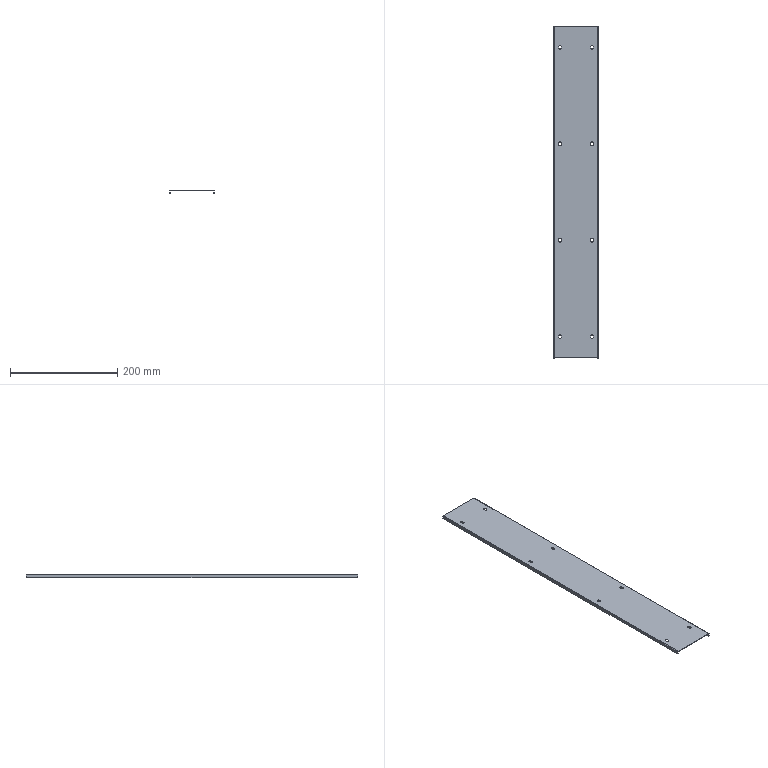Part | STEP file | 1 solid | 58 faces | box 83 x 620 x 6 mm | volume 57149 mm3 | plane 34 | cylinder 24 | commonest cylinder face diameters 4.5 x16 2 x4 0.1 x2 2.1 x2